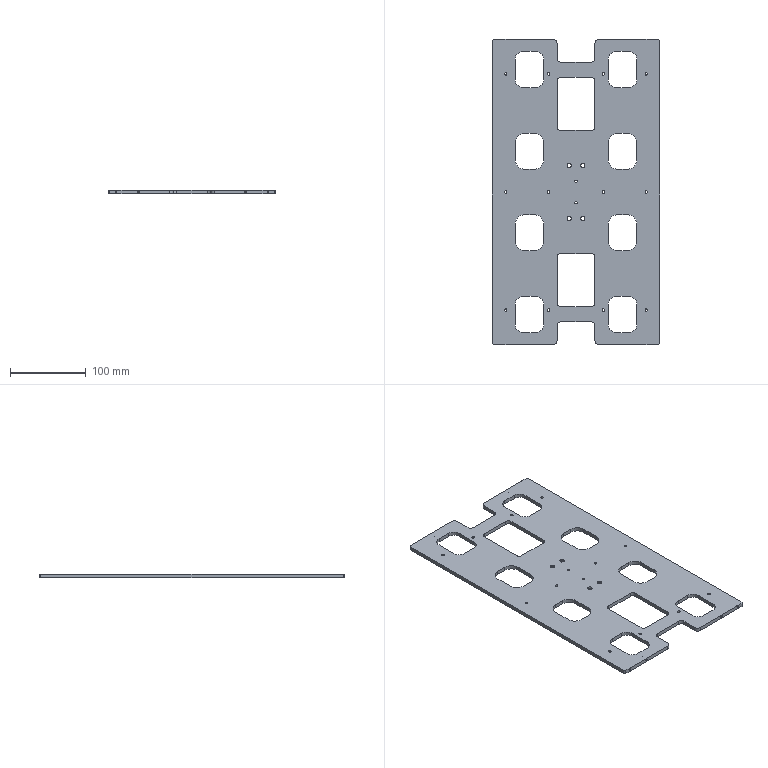Part | STEP file | 11-FG-SZ02711 | 1 solid | 182 faces | box 220 x 402 x 5 mm | volume 323652 mm3 | cylinder 100 | plane 58 | cone 24 | commonest cylinder face diameters 3.3 x24 2.5 x16 10 x16 20 x16 24.38 x16 5.5 x8